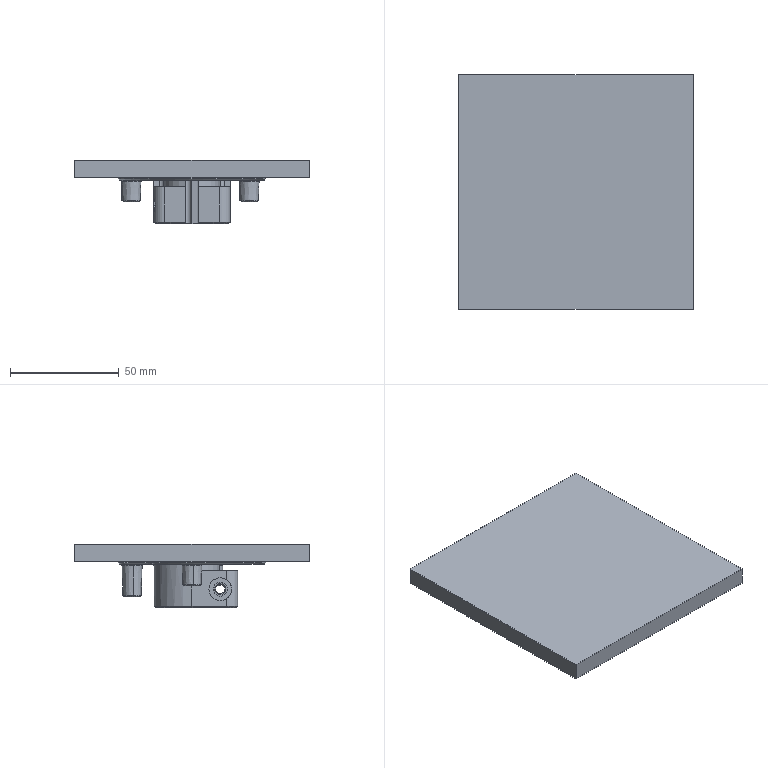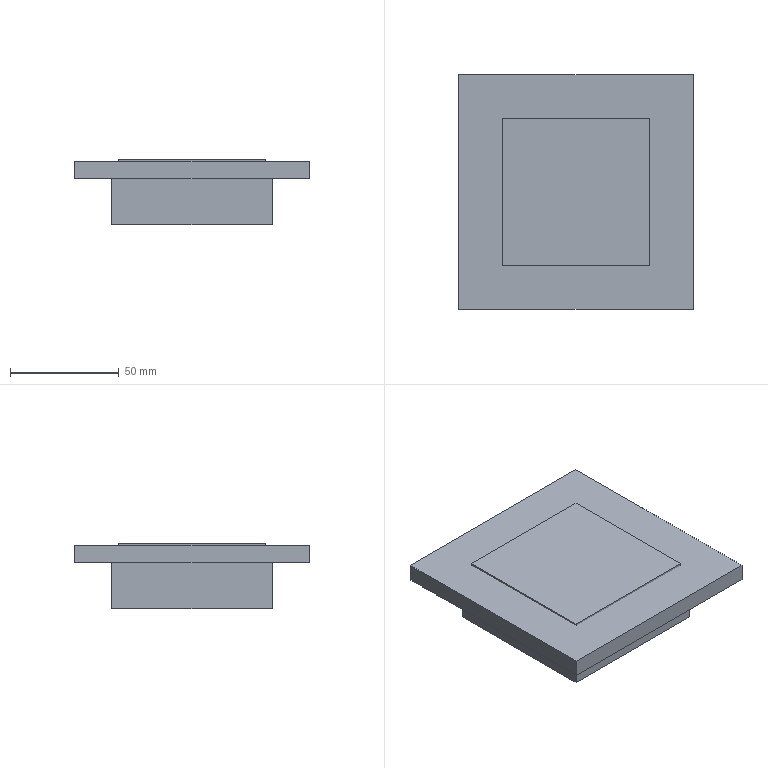CAM job | NX | 3-axis milling, drilling | part box 108 x 108 x 29 mm | stock box 108 x 108 x 30 mm
Tools:
number,name,description,diameter,corner_radius,flute_length,length,flutes
3,D63,Milling Tool-5 Parameters,63.0,0.0,50.0,75.0,2
1,D6A45,Milling Tool-5 Parameters,6.0,0.0,3.0,3.0,2
11,5.1ZT,Drilling Tool,5.1,0.0,35.0,50.0,2
12,3.0ZT,Drilling Tool,3.0,0.0,35.0,50.0,2
4,D10,Milling Tool-5 Parameters,10.0,0.0,50.0,75.0,2
16,D6JING,Milling Tool-5 Parameters,6.0,0.0,50.0,75.0,2
17,D3,Milling Tool-5 Parameters,3.0,0.0,50.0,75.0,2
15,D4,Milling Tool-5 Parameters,4.0,0.0,50.0,75.0,2
7,D3R0.5,Milling Tool-5 Parameters,3.0,0.5,50.0,75.0,2
13,4.2ZT,Drilling Tool,4.2,0.0,35.0,80.0,2
20,6.5ZT,Drilling Tool,6.5,0.0,35.0,80.0,2
Operations:
program,operation,operation_type,tool,method,geometry_group,spindle_rpm,surface_speed,feed_per_tooth,feed_cut,feed_plunge,cut_length_mm,path_length_mm,cut_time_min,machine_time_min
1,FLOOR_WALL_COPY,VolumeBased25DMillingOperation,D63,METHOD,A,6500.0,1286.0,0.0962,1250.0,100.0,316.793,370.793,0.2534,0.2588
1,DRILLING_COPY_1,Operation,D6A45,METHOD,A,5000.0,94.0,0.025,250.0,0.0,20.0,212.939,0.08,0.0993
1,DRILLING_COPY_1_COPY,Operation,5.1ZT,METHOD,A,2000.0,20.0,0.0625,250.0,0.0,68.097,300.427,0.2724,0.2956
1,DRILLING_COPY_1_COPY_COPY_1,Operation,5.1ZT,METHOD,A,2000.0,20.0,0.0625,250.0,0.0,31.032,122.064,0.1241,0.1332
1,DRILLING_COPY_1_COPY_COPY,Operation,3.0ZT,METHOD,A,2122.0,20.0,0.0353,150.0,0.0,30.401,120.803,0.2027,0.2117
1,ADAPTIVE_MILLING_COPY,CavityMilling,D10,METHOD,A,9500.0,298.0,0.1842,3500.0,1000.0,10117.979,10564.892,4.274,4.318
1,ZLEVEL_PROFILE_COPY_COPY_COPY_1_COPY_COPY_1,ZLevelMilling,D6JING,METHOD,A,9500.0,89.0,0.0789,1500.0,1000.0,884.83,1473.239,0.6551,0.7139
1,ZLEVEL_PROFILE_1_COPY,ZLevelMilling,D6JING,METHOD,A,9500.0,298.0,0.0526,1000.0,100.0,613.701,904.526,0.6137,0.6428
1,ZLEVEL_PROFILE_COPY,ZLevelMilling,D6JING,METHOD,A,9500.0,179.0,0.1053,2000.0,1000.0,1175.703,1322.43,0.6165,0.6312
1,ZLEVEL_PROFILE_COPY_COPY,ZLevelMilling,D6JING,METHOD,A,9500.0,179.0,0.1053,2000.0,1000.0,1797.579,1863.579,0.9131,0.9197
1,ZLEVEL_PROFILE_1_COPY_COPY,ZLevelMilling,D6JING,METHOD,A,9500.0,298.0,0.0526,1000.0,100.0,113.519,187.519,0.1135,0.1209
1,ZLEVEL_PROFILE_COPY_COPY_COPY_1_COPY,ZLevelMilling,D4,METHOD,A,9500.0,89.0,0.0789,1500.0,1000.0,364.806,791.628,0.2715,0.3142
1,ZLEVEL_PROFILE_COPY_COPY_COPY_1_COPY_COPY,ZLevelMilling,D3,METHOD,A,9500.0,89.0,0.0447,850.0,1000.0,1727.763,2297.417,2.008,2.065
1,ZLEVEL_PROFILE_COPY_COPY_COPY,ZLevelMilling,D3R0.5,METHOD,A,9500.0,119.0,0.1053,2000.0,1000.0,1937.685,2203.384,0.9995,1.026
1,ZLEVEL_PROFILE_COPY_COPY_COPY_COPY,ZLevelMilling,D3R0.5,METHOD,A,9500.0,119.0,0.1053,2000.0,1000.0,1419.858,1479.417,0.7108,0.7168
1,11,ZLevelMilling,D6A45,METHOD,A,9500.0,179.0,0.0526,1000.0,100.0,133.829,189.829,0.1338,0.1394
1,11_COPY_COPY,ZLevelMilling,D6A45,METHOD,A,9500.0,179.0,0.0526,1000.0,100.0,246.783,302.783,0.2468,0.2524
2,FLOOR_WALL_COPY_COPY,VolumeBased25DMillingOperation,D63,METHOD,B,6500.0,1286.0,0.0962,1250.0,100.0,1583.995,2004.291,1.267,1.309
2,FLOOR_WALL_COPY_COPY_1,VolumeBased25DMillingOperation,D63,METHOD,B,6500.0,1286.0,0.0962,1250.0,100.0,316.793,370.793,0.2534,0.2588
2,CAVITY_MILL,CavityMilling,D10,METHOD,B,9500.0,298.0,0.1316,2500.0,1000.0,12692.025,12824.692,5.263,5.276
2,CAVITY_MILL_COPY,CavityMilling,D6JING,METHOD,B,9500.0,179.0,0.0789,1500.0,1000.0,3874.53,5351.71,2.781,2.929
2,CAVITY_MILL_COPY_COPY,CavityMilling,D4,METHOD,B,9500.0,119.0,0.0737,1400.0,1000.0,3108.138,4240.386,2.314,2.427
2,ZLEVEL_PROFILE_1_COPY_COPY_COPY,ZLevelMilling,D4,METHOD,B,9500.0,298.0,0.0526,1000.0,100.0,157.344,235.344,0.1573,0.1651
2,FLOOR_WALL_1_COPY_1,VolumeBased25DMillingOperation,D4,METHOD,B,9500.0,298.0,0.0632,1200.0,1000.0,1524.228,2495.857,1.275,1.372
2,ZLEVEL_PROFILE_COPY_COPY_COPY_COPY_1,ZLevelMilling,D3R0.5,METHOD,B,9500.0,119.0,0.1053,2000.0,1000.0,14702.006,15068.485,7.382,7.418
2,11_COPY,ZLevelMilling,D6A45,METHOD,B,9500.0,179.0,0.0526,1000.0,100.0,216.538,272.538,0.2165,0.2221
2,11_COPY_COPY_1,ZLevelMilling,D6A45,METHOD,B,9500.0,179.0,0.0526,1000.0,100.0,58.044,195.621,0.058,0.0718
2,11_COPY_COPY_1_COPY,ZLevelMilling,D6A45,METHOD,B,9500.0,179.0,0.0526,1000.0,100.0,116.199,548.34,0.1162,0.1594
2,11_COPY_COPY_1_COPY_COPY,ZLevelMilling,D6A45,METHOD,B,9500.0,179.0,0.0526,1000.0,100.0,225.627,642.801,0.2256,0.2673
2,DRILLING,HoleDrilling,D6A45,METHOD,B,5000.0,94.0,0.025,250.0,0.0,10.0,49.06,0.02,0.0239
2,DRILLING_COPY,HoleDrilling,4.2ZT,METHOD,B,2000.0,26.0,0.025,100.0,0.0,871.524,908.784,0.3976,0.4013
2,DRILLING_COPY_COPY,HoleDrilling,6.5ZT,METHOD,B,2000.0,26.0,0.025,100.0,0.0,231.906,271.466,0.1995,0.2035
2,HOLE_MILLING,CylinderMilling,D6JING,METHOD,B,9500.0,179.0,0.0763,1450.0,100.0,275.834,327.854,0.1902,0.1954
3,CAVITY_MILL_COPY_1,CavityMilling,D6JING,METHOD,C,9500.0,298.0,0.1316,2500.0,1000.0,11639.712,11973.749,4.924,4.958
3,FLOOR_WALL_1_COPY_1_COPY,VolumeBased25DMillingOperation,D6JING,METHOD,C,9500.0,298.0,0.0632,1200.0,1000.0,1068.909,1168.327,0.8918,0.9026
3,11_COPY_1,ZLevelMilling,D6A45,METHOD,C,9500.0,179.0,0.0526,1000.0,100.0,237.657,293.657,0.2377,0.2433
3,刀补16,VolumeBased25DMillingOperation,D6JING,METHOD,C,9500.0,298.0,0.0632,1200.0,1000.0,222.092,287.092,0.1857,0.1922